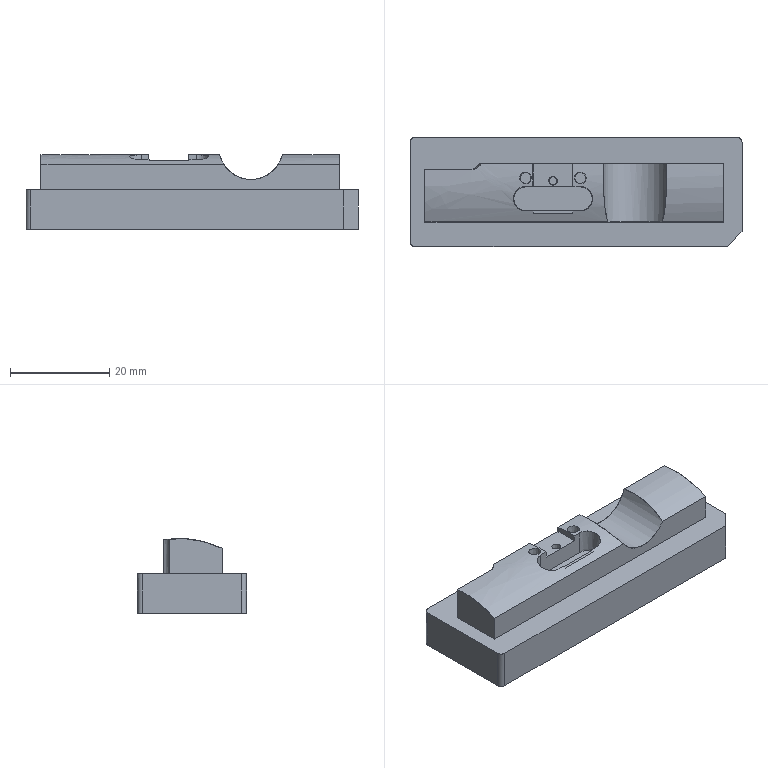NC program | PowerMill | posted with a generic post | part box 67 x 22 x 15.086 mm
Lines 1 to 1040 of 148586:
%
O0001
N104 ( POWERMILL CB  : 2026004.0)
N105 ( POST VER      : 2026.0.0.5161)
N106 ( OPTION FILE   : FANUC)
N107 ( OUTPUT WORKPLANE : WORLD)
N108 (  )
N109 ( TOOL LIST )
N110 (---------------------------------------)
N111 ( NO. | ID        | DIA.| TIP RAD|LENGTH)
N112 (---------------------------------------)
N113 (    1|D10C_1_1   |10.0 |  0.0   |70.52 )
N114 (   15|D3C_2_1    | 3.0 |  0.0   |62.16 )
N115 (   27|D1C_2_1    | 1.0 |  0.0   |60.24 )
N116 (    3|D10_1_1    |10.0 |  0.0   |70.24 )
N117 (   22|R1.5_1_1   | 3.0 |  1.5   |60.28 )
N118 (   10|D3_1_1_1_2 | 3.0 |  0.0   | 62.2 )
N119 (    8|D1_1_1     | 1.0 |  0.0   |60.28 )
N120 (   13|TEXT_D4_1_1| 4.0 |  0.3   |62.36 )
N121 (---------------------------------------)
N122 (  )
N123 ( NUMBER OF TOOLPATHS: 17.0 )
N124 ( ESTIMATED PROGRAM DURATION: 0 HOURS 22 MIN 14 SEC)
N125 (  )
N126 G00 G21 G80 G40 G17
N127 G90
N128 G54
N129 G53 Z0.0
N130 (---------------)
N131 ( START TOOLPATH : 粗公开粗01-扫面平行-D10C )
N132 (---------------)
N133 ( TOOL NO.    :1 )
N134 ( TOOL TYPE   : ENDMILL)
N135 ( TOOL ID     : D10C_1_1)
N136 ( TOOL DIA    : 10.0 LENGTH 70.52)
N137 T1
N138 M6
N139 S8000 M03
N140 G00 G90 X0.0 Y0.0
N141 G43 Z10.2 H1
N142
N143 G05 P10000 R4
N144 X41.15 Y13.65
N145 Z1.1975
N146 G01 Z-0.0025 F6000.0
N147 X36.15 F10000.0
N148 X-36.15
N149 Y8.19
N150 X36.15
N151 Y2.73
N152 X-36.15
N153 Y-2.73
N154 X36.15
N155 Y-8.19
N156 X-36.15
N157 Y-13.65
N158 X36.15
N159 X41.15
N160 Z-0.205
N161 X36.15
N162 X-36.15
N163 Y-8.19
N164 X36.15
N165 Y-2.73
N166 X-36.15
N167 Y2.73
N168 X36.15
N169 Y8.19
N170 X-36.15
N171 Y13.65
N172 X36.15
N173 X41.15
N174 G00 Z10.2
N175 G05 P0
N176 (---------------)
N177 ( END TOOLPATH : 粗公开粗01-扫面平行-D10C )
N178 (---------------)
N179 ( START TOOLPATH : 粗公开粗01-外形偏置-D10C )
N180 (---------------)
N181 G00 X-0.3595 Y-0.0315 Z9.7955
N182 G05 P10000 R4
N183 X42.682 Y10.5169
N184 Z0.6351
N185 G01 Z-0.5649 F6000.0
N186 X42.1545 F10000.0
N187 G03 X37.407 Y5.7694 I0.0 J-4.7475
N188 G01 Y-12.713
N189 G02 X36.407 Y-13.713 I-1.0 J0.0
N190 G01 X-4.6615
N191 Y-9.213
N192 Y-13.713
N193 X-37.126
N194 G02 X-38.126 Y-12.713 I0.0 J1.0
N195 G01 Y12.65
N196 G02 X-37.126 Y13.65 I1.0 J0.0
N197 G01 X36.407
N198 G02 X37.407 Y12.65 I0.0 J-1.0
N199 G01 Y5.7694
N200 X34.9091 Y5.7692
N201 X34.9095 Y-0.4182
N202 X34.902 Y-1.1916
N203 X34.8314 Y-1.8088
N204 X34.5777 Y-2.7385
N205 X34.2095 Y-3.5119
N206 X34.058 Y-3.7528
N207 X33.6575 Y-4.2853
N208 X33.2846 Y-4.6749
N209 X32.8237 Y-5.0588
N210 X32.5111 Y-5.273
N211 X31.7377 Y-5.6689
N212 X31.2876 Y-5.8322
N213 X30.9643 Y-5.9218
N214 X30.1908 Y-6.0524
N215 X29.4174 Y-6.0514
N216 X28.644 Y-6.0081
N217 X22.4566 Y-6.0108
N218 X22.4537
N219 X17.816 Y-6.0659
N220 X17.0426 Y-5.9479
N221 X16.2692 Y-5.7099
N222 X15.4957 Y-5.3238
N223 X15.101 Y-5.0588
N224 X14.7223 Y-4.747
N225 X14.2769 Y-4.2853
N226 X13.9489 Y-3.8691
N227 X13.7229 Y-3.5119
N228 X13.3569 Y-2.7385
N229 X13.1755 Y-2.1508
N230 X13.0336 Y-1.1916
N231 X13.0168 Y-0.4182
N232 X13.0199 Y5.7692
N233 X13.0201 Y5.7722
N234 X10.7908 Y5.7692
N235 X10.7971 Y1.1286
N236 X10.7768 Y-1.1916
N237 X10.6755 Y-1.9651
N238 X10.4515 Y-2.7385
N239 X10.0818 Y-3.5197
N240 X9.5319 Y-4.2853
N241 X9.3083 Y-4.5323
N242 X8.5349 Y-5.1785
N243 X7.7615 Y-5.6129
N244 X7.1733 Y-5.8322
N245 X6.9881 Y-5.8926
N246 X6.2146 Y-6.039
N247 X5.4412 Y-6.0733
N248 X3.1209 Y-6.0724
N249 X2.3475 Y-5.9868
N250 X1.7218 Y-5.8322
N251 X0.8006 Y-5.4335
N252 X0.0272 Y-4.9161
N253 X-0.6151 Y-4.2853
N254 X-0.6631 Y-4.2274
N255 G03 X-0.9979 Y-4.049 I-0.385 J-0.319
N256 G01 X-1.5196 Y-3.9963
N257 X-2.2931 Y-3.7998
N258 X-2.9778 Y-3.5119
N259 X-3.8399 Y-2.9592
N260 X-4.1006 Y-2.7385
N261 X-4.2919 Y-2.5355
N262 G03 X-4.999 Y-2.5149 I-0.3639 J-0.343
N263 G01 X-5.3868 Y-2.8809
N264 X-6.1602 Y-3.4124
N265 X-6.9336 Y-3.7663
N266 X-7.7071 Y-3.9745
N267 X-8.2974 Y-4.0446
N268 G03 X-8.6235 Y-4.2222 I0.059 J-0.4965
N269 G01 X-8.6758 Y-4.2853
N270 X-9.2539 Y-4.8636
N271 X-9.5052 Y-5.0588
N272 X-10.0273 Y-5.3961
N273 X-10.8008 Y-5.7558
N274 X-11.5742 Y-5.977
N275 X-12.3476 Y-6.0711
N276 X-22.4022 Y-6.0455
N277 X-29.363 Y-6.0403
N278 X-30.9098 Y-6.0527
N279 X-31.6833 Y-5.9206
N280 X-32.014 Y-5.8322
N281 X-32.4567 Y-5.6676
N282 X-33.2301 Y-5.2723
N283 X-33.5386 Y-5.0588
N284 X-34.0036 Y-4.6734
N285 X-34.3712 Y-4.2853
N286 X-34.777 Y-3.755
N287 X-34.9267 Y-3.5119
N288 X-35.2947 Y-2.7385
N289 X-35.518 Y-1.9651
N290 X-35.6189 Y-1.1916
N291 X-35.6268 Y4.2223
N292 X-35.6035 Y4.9958
N293 X-35.5504 Y5.391
N294 X-35.4698 Y5.7692
N295 X-35.2075 Y6.5426
N296 X-34.7935 Y7.3161
N297 X-34.177 Y8.0895
N298 X-34.0036 Y8.2604
N299 X-33.2301 Y8.8597
N300 X-32.4567 Y9.2617
N301 X-31.6833 Y9.5142
N302 X-30.9437 Y9.6363
N303 X-30.1364 Y9.6575
N304 X-22.6114
N305 X-22.4647 Y9.6796
N306 X-22.3309 Y9.7437
N307 X-21.6287 Y10.2196
N308 X-21.2529 Y10.4098
N309 X-20.8553 Y10.568
N310 X-20.0819 Y10.7731
N311 X-19.3084 Y10.8552
N312 X-10.0273 Y10.8575
N313 X-8.4805 Y10.8536
N314 X-7.7071 Y10.7648
N315 X-6.9336 Y10.5524
N316 X-6.5839 Y10.4098
N317 X-6.1602 Y10.1987
N318 X-5.3868 Y9.6623
N319 X-4.9839 Y9.2936
N320 G03 X-4.288 Y9.3138 I0.3376 J0.3689
N321 G01 X-3.9741 Y9.6363
N322 X-3.8399 Y9.7461
N323 X-3.0665 Y10.2523
N324 X-2.7447 Y10.4098
N325 X-2.2931 Y10.5865
N326 X-1.5196 Y10.7826
N327 X-0.7462 Y10.8565
N328 X5.4412 Y10.8575
N329 X6.2146 Y10.8253
N330 X6.9881 Y10.6781
N331 X7.7416 Y10.4098
N332 X8.5349 Y9.9667
N333 X8.971 Y9.6363
N334 X9.3083 Y9.3226
N335 X9.7115 Y8.8629
N336 X10.0818 Y8.3149
N337 X10.2073 Y8.0895
N338 X10.5336 Y7.3161
N339 X10.7231 Y6.5426
N340 X10.7908 Y5.7692
N341 X13.0201 Y5.7722
N342 X13.0877 Y6.5426
N343 X13.1755 Y6.9645
N344 X13.2771 Y7.3161
N345 X13.6034 Y8.0895
N346 X13.9489 Y8.6575
N347 X14.0993 Y8.8629
N348 X14.7223 Y9.5329
N349 X15.4957 Y10.1085
N350 X16.2692 Y10.4935
N351 X17.0426 Y10.7327
N352 X17.816 Y10.8431
N353 X18.5894 Y10.8575
N354 X29.4174
N355 X30.1908 Y10.8394
N356 X30.9643 Y10.7146
N357 X31.7377 Y10.4624
N358 X32.5111 Y10.0608
N359 X33.0892 Y9.6363
N360 X33.2846 Y9.462
N361 X33.8296 Y8.8629
N362 X34.058 Y8.544
N363 X34.3255 Y8.0895
N364 X34.6519 Y7.3161
N365 X34.8314 Y6.601
N366 X34.9091 Y5.7692
N367 X37.407 Y5.7694
N368 G00 Z3.3752
N369 G01 X42.682 Y10.5169
N370 G00 Z0.3252
N371 G01 Z-0.8748 F6000.0
N372 X42.1545 F10000.0
N373 G03 X37.407 Y5.7694 I0.0 J-4.7475
N374 G01 Y5.7693
N375 X34.9091 Y5.7692
N376 X34.9093 Y2.0706
N377 X34.9094 Y-0.4182
N378 Y-0.4219
N379 X34.9095 Y-1.9651
N380 X34.8916 Y-2.7385
N381 X34.8314 Y-3.207
N382 X34.7668 Y-3.5119
N383 X34.5157 Y-4.2853
N384 X34.116 Y-5.0588
N385 X33.5168 Y-5.8322
N386 X33.2846 Y-6.068
N387 X32.5971 Y-6.6056
N388 X31.7377 Y-7.0685
N389 X30.9643 Y-7.3208
N390 X30.6654 Y-7.3791
N391 X30.1908 Y-7.4432
N392 X28.644 Y-7.4283
N393 X22.4566 Y-7.4306
N394 X22.4547
N395 X17.816 Y-7.4676
N396 X17.0426 Y-7.3692
N397 X16.2692 Y-7.1465
N398 X15.4957 Y-6.7804
N399 X15.2212 Y-6.6056
N400 X14.7223 Y-6.2304
N401 X14.3092 Y-5.8322
N402 X13.9489 Y-5.4021
N403 X13.715 Y-5.0588
N404 X13.317 Y-4.2853
N405 X13.1755 Y-3.9008
N406 X13.0677 Y-3.5119
N407 X12.9462 Y-2.7385
N408 X12.9179 Y-1.9651
N409 X12.9181 Y4.2223
N410 X12.9141 Y5.7532
N411 X10.8966 Y5.7692
N412 X10.8905 Y4.9958
N413 X10.8922 Y-1.9651
N414 X10.864 Y-2.7385
N415 X10.7422 Y-3.5119
N416 X10.4904 Y-4.2853
N417 X10.0818 Y-5.0809
N418 X9.499 Y-5.8322
N419 X9.3083 Y-6.0291
N420 X8.5875 Y-6.6056
N421 X7.7615 Y-7.0549
N422 X6.9881 Y-7.3168
N423 X6.7042 Y-7.3791
N424 X6.2146 Y-7.4503
N425 X5.4412 Y-7.4734
N426 X3.1209 Y-7.472
N427 X2.3475 Y-7.4118
N428 X1.5741 Y-7.2306
N429 X0.8006 Y-6.9135
N430 X0.0272 Y-6.4409
N431 X-0.7462 Y-5.7134
N432 X-1.2329 Y-5.0588
N433 X-1.5196 Y-4.5318
N434 X-1.6599 Y-4.1825
N435 G03 X-1.9896 Y-3.8871 I-0.464 J-0.1863
N436 G01 X-2.2931 Y-3.8026
N437 X-2.9826 Y-3.5119
N438 X-3.8399 Y-2.9615
N439 X-4.1029 Y-2.7385
N440 X-4.2909 Y-2.5388
N441 G03 X-4.9983 Y-2.5178 I-0.3641 J-0.3426
N442 G01 X-5.3868 Y-2.8846
N443 X-6.1602 Y-3.4163
N444 X-6.9336 Y-3.7695
N445 X-7.2951 Y-3.8753
N446 G03 X-7.6232 Y-4.1805 I0.1405 J-0.4799
N447 G01 X-7.6622 Y-4.2853
N448 X-8.0571 Y-5.0588
N449 X-8.4805 Y-5.6386
N450 X-8.6556 Y-5.8322
N451 X-9.2539 Y-6.3874
N452 X-10.0273 Y-6.88
N453 X-10.8008 Y-7.21
N454 X-11.4341 Y-7.3791
N455 X-12.3476 Y-7.4716
N456 X-17.7616 Y-7.4491
N457 X-29.363 Y-7.4299
N458 X-30.9098 Y-7.4433
N459 X-31.6833 Y-7.3204
N460 X-32.4567 Y-7.0677
N461 X-33.2301 Y-6.6652
N462 X-34.0036 Y-6.0664
N463 X-34.2347 Y-5.8322
N464 X-34.777 Y-5.1473
N465 X-35.233 Y-4.2853
N466 X-35.4849 Y-3.5119
N467 X-35.609 Y-2.7385
N468 X-35.6268 Y-1.9651
N469 Y4.2223
N470 X-35.6035 Y4.9958
N471 X-35.5504 Y5.391
N472 X-35.4698 Y5.7692
N473 X-35.2075 Y6.5426
N474 X-34.7935 Y7.3161
N475 X-34.177 Y8.0895
N476 X-34.0036 Y8.2604
N477 X-33.2301 Y8.8597
N478 X-32.4567 Y9.2617
N479 X-31.6833 Y9.5142
N480 X-30.9437 Y9.6363
N481 X-30.1364 Y9.6575
N482 X-22.6283
N483 X-22.4813 Y9.6796
N484 X-22.3473 Y9.744
N485 X-21.6287 Y10.2321
N486 X-21.2696 Y10.4098
N487 X-20.8553 Y10.5737
N488 X-20.0819 Y10.776
N489 X-19.3084 Y10.8557
N490 X-10.0273 Y10.8575
N491 X-8.4805 Y10.8537
N492 X-7.7071 Y10.765
N493 X-6.9336 Y10.5529
N494 X-6.5808 Y10.4098
N495 X-6.1602 Y10.1997
N496 X-5.3868 Y9.6652
N497 X-4.9844 Y9.295
N498 G03 X-4.2876 Y9.3143 I0.3385 J0.368
N499 G01 X-3.9741 Y9.6363
N500 X-3.8399 Y9.7461
N501 X-3.0665 Y10.2523
N502 X-2.7447 Y10.4098
N503 X-2.2931 Y10.5865
N504 X-1.5196 Y10.7826
N505 X-0.7462 Y10.8565
N506 X5.4412 Y10.8575
N507 X6.2146 Y10.835
N508 X6.9881 Y10.7046
N509 X7.7615 Y10.4461
N510 X8.5349 Y10.0363
N511 X9.0767 Y9.6363
N512 X9.3083 Y9.4271
N513 X9.8176 Y8.8629
N514 X10.0818 Y8.4876
N515 X10.3131 Y8.0895
N516 X10.6394 Y7.3161
N517 X10.8289 Y6.5426
N518 X10.8966 Y5.7692
N519 X12.9141 Y5.7532
N520 Y5.7692
N521 X12.9819 Y6.5426
N522 X13.1714 Y7.3161
N523 X13.4975 Y8.0895
N524 X13.9489 Y8.8032
N525 X14.7223 Y9.6264
N526 X15.4957 Y10.1711
N527 X15.9632 Y10.4098
N528 X16.2692 Y10.5339
N529 X17.0426 Y10.7542
N530 X17.816 Y10.8515
N531 X18.5894 Y10.8575
N532 X29.4174
N533 X30.1908 Y10.8394
N534 X30.9643 Y10.7146
N535 X31.7377 Y10.4624
N536 X32.5111 Y10.0608
N537 X33.0892 Y9.6363
N538 X33.2846 Y9.462
N539 X33.8296 Y8.8629
N540 X34.058 Y8.544
N541 X34.3255 Y8.0895
N542 X34.6519 Y7.3161
N543 X34.8314 Y6.601
N544 X34.9091 Y5.7692
N545 X37.407 Y5.7693
N546 Y-12.713
N547 G02 X36.407 Y-13.713 I-1.0 J0.0
N548 G01 X-37.126
N549 G02 X-38.126 Y-12.713 I0.0 J1.0
N550 G01 Y12.65
N551 G02 X-37.126 Y13.65 I1.0 J0.0
N552 G01 X36.407
N553 G02 X37.407 Y12.65 I0.0 J-1.0
N554 G01 Y5.7694
N555 G00 Z3.0653
N556 G01 X42.682 Y10.5169
N557 G00 Z0.0153
N558 G01 Z-1.1847 F6000.0
N559 X42.1545 F10000.0
N560 G03 X37.407 Y5.7694 I0.0 J-4.7475
N561 G01 Y5.7687
N562 X34.9091 Y5.7692
N563 X34.909 Y5.5281
N564 X34.9092 Y2.0706
N565 X34.9094 Y-0.4182
N566 Y-0.4219
N567 Y-1.9651
N568 X34.9076 Y-2.0433
N569 X34.9074 Y-3.5119
N570 X34.8314 Y-4.2796
N571 X34.6301 Y-5.0588
N572 X34.2915 Y-5.8322
N573 X34.058 Y-6.2197
N574 X33.7768 Y-6.6056
N575 X33.2846 Y-7.1406
N576 X33.012 Y-7.3791
N577 X32.5111 Y-7.7394
N578 X31.7071 Y-8.1525
N579 X30.9643 Y-8.3932
N580 X30.1908 Y-8.517
N581 X17.816 Y-8.5325
N582 X17.0426 Y-8.4525
N583 X16.2692 Y-8.2483
N584 X15.4957 Y-7.9062
N585 X14.7223 Y-7.387
N586 X13.9464 Y-6.6056
N587 X13.4325 Y-5.8322
N588 X13.1755 Y-5.2828
N589 X13.0938 Y-5.0588
N590 X12.8926 Y-4.2853
N591 X12.8097 Y-3.5119
N592 X12.8062 Y-2.7385
N593 X12.8116 Y4.2223
N594 X12.808 Y5.7687
N595 X11.0043 Y5.7692
N596 X11.0016 Y-3.5119
N597 X10.9187 Y-4.2853
N598 X10.7181 Y-5.0588
N599 X10.3789 Y-5.8322
N600 X10.0818 Y-6.3179
N601 X9.8656 Y-6.6056
N602 X9.3083 Y-7.2001
N603 X9.0981 Y-7.3791
N604 X8.5349 Y-7.7793
N605 X7.792 Y-8.1525
N606 X6.9881 Y-8.4077
N607 X6.2146 Y-8.5185
N608 X2.3475 Y-8.5338
N609 X1.5741 Y-8.4902
N610 X0.8006 Y-8.325
N611 X0.0272 Y-8.0304
N612 X-0.7462 Y-7.5736
N613 X-1.5196 Y-6.8894
N614 X-1.7538 Y-6.6056
N615 X-2.2707 Y-5.8322
N616 X-2.6045 Y-5.0588
N617 X-2.8054 Y-4.2853
N618 X-2.8511 Y-3.8329
N619 G03 X-3.0745 Y-3.465 I-0.4975 J-0.0502
N620 G01 X-3.8399 Y-2.9633
N621 X-4.1047 Y-2.7385
N622 X-4.2897 Y-2.5417
N623 G03 X-4.9973 Y-2.5206 I-0.3643 J-0.3425
N624 G01 X-5.3868 Y-2.8884
N625 X-6.1602 Y-3.4197
N626 X-6.1671 Y-3.4233
N627 G03 X-6.4319 Y-3.815 I0.2326 J-0.4426
N628 G01 X-6.48 Y-4.2853
N629 X-6.6818 Y-5.0588
N630 X-7.0209 Y-5.8322
N631 X-7.5341 Y-6.6056
N632 X-7.7071 Y-6.8087
N633 X-8.2994 Y-7.3791
N634 X-8.4805 Y-7.518
N635 X-9.2539 Y-7.9992
N636 X-9.5968 Y-8.1525
N637 X-10.0273 Y-8.3074
N638 X-10.8008 Y-8.4834
N639 X-11.5742 Y-8.5386
N640 X-30.9098 Y-8.517
N641 X-31.6833 Y-8.3928
N642 X-32.4567 Y-8.1398
N643 X-33.2301 Y-7.7383
N644 X-33.7288 Y-7.3791
N645 X-34.0036 Y-7.1391
N646 X-34.4956 Y-6.6056
N647 X-34.777 Y-6.2168
N648 X-35.0078 Y-5.8322
N649 X-35.3472 Y-5.0588
N650 X-35.5474 Y-4.2853
N651 X-35.6242 Y-3.5119
N652 X-35.6247 Y-2.0542
N653 X-35.6267 Y-1.9651
N654 Y4.0618
N655 X-35.6268 Y4.2223
N656 X-35.6035 Y4.9958
N657 X-35.5504 Y5.391
N658 X-35.4698 Y5.7692
N659 X-35.2075 Y6.5426
N660 X-34.7935 Y7.3161
N661 X-34.177 Y8.0895
N662 X-34.0036 Y8.2604
N663 X-33.2301 Y8.8597
N664 X-32.4567 Y9.2617
N665 X-31.6833 Y9.5142
N666 X-30.9437 Y9.6363
N667 X-30.1364 Y9.6575
N668 X-22.6439
N669 X-22.4974 Y9.6795
N670 X-22.3638 Y9.7434
N671 X-21.6287 Y10.2407
N672 X-21.2859 Y10.4098
N673 X-20.8553 Y10.5793
N674 X-20.0819 Y10.7789
N675 X-19.3084 Y10.8561
N676 X-10.0273 Y10.8575
N677 X-8.4805 Y10.8538
N678 X-7.7071 Y10.7653
N679 X-6.9336 Y10.5534
N680 X-6.5776 Y10.4098
N681 X-6.1602 Y10.2004
N682 X-5.3868 Y9.6681
N683 X-5.1713 Y9.4796
N684 X-5.0894 Y9.3916
N685 X-4.9844 Y9.295
N686 G03 X-4.3094 Y9.2932 I0.3385 J0.368
N687 G01 X-4.3021 Y9.3002
N688 X-4.2949 Y9.3074
N689 X-3.9741 Y9.6363
N690 X-3.8399 Y9.7462
N691 X-3.0665 Y10.2524
N692 X-2.7448 Y10.4098
N693 X-2.2931 Y10.5866
N694 X-1.5196 Y10.7827
N695 X-0.7462 Y10.8565
N696 X5.4412 Y10.8575
N697 X6.2146 Y10.8448
N698 X6.9881 Y10.7311
N699 X7.7615 Y10.4918
N700 X8.5349 Y10.1042
N701 X9.1846 Y9.6363
N702 X9.9237 Y8.8629
N703 X10.0818 Y8.6476
N704 X10.4197 Y8.0895
N705 X10.7467 Y7.3161
N706 X10.8552 Y6.9347
N707 X10.9349 Y6.5426
N708 X11.0043 Y5.7692
N709 X12.808 Y5.7687
N710 Y5.7692
N711 X12.8754 Y6.5426
N712 X13.0646 Y7.3161
N713 X13.1755 Y7.6201
N714 X13.3915 Y8.0895
N715 X13.886 Y8.8629
N716 X14.6274 Y9.6363
N717 X15.4957 Y10.2311
N718 X15.8572 Y10.4098
N719 X16.2692 Y10.5744
N720 X17.0426 Y10.7756
N721 X17.816 Y10.8556
N722 X18.3645 Y10.8557
N723 X18.5894 Y10.8575
N724 X29.0893
N725 X29.4174
N726 X30.1908 Y10.8395
N727 X30.9643 Y10.7146
N728 X31.7377 Y10.4624
N729 X32.5111 Y10.0608
N730 X33.0892 Y9.6363
N731 X33.2846 Y9.462
N732 X33.8297 Y8.8629
N733 X34.058 Y8.544
N734 X34.3255 Y8.0895
N735 X34.6519 Y7.3161
N736 X34.8314 Y6.601
N737 X34.9091 Y5.7692
N738 X37.407 Y5.7687
N739 Y-12.713
N740 G02 X36.407 Y-13.713 I-1.0 J0.0
N741 G01 X-37.126
N742 G02 X-38.126 Y-12.713 I0.0 J1.0
N743 G01 Y12.65
N744 G02 X-37.126 Y13.65 I1.0 J0.0
N745 G01 X36.407
N746 G02 X37.407 Y12.65 I0.0 J-1.0
N747 G01 Y5.7694
N748 G00 Z2.7554
N749 G01 X42.682 Y10.5169
N750 G00 Z-0.2946
N751 G01 Z-1.4946 F6000.0
N752 X42.1545 F10000.0
N753 G03 X37.407 Y5.7694 I0.0 J-4.7475
N754 G01 Y5.7693
N755 X34.9091 Y5.7692
N756 X34.9092 Y2.2259
N757 Y2.0706
N758 X34.9093 Y-0.4182
N759 Y-0.4219
N760 X34.9094 Y-1.9651
N761 X34.9093 Y-1.9708
N762 Y-4.2853
N763 X34.8441 Y-5.0588
N764 X34.6584 Y-5.8322
N765 X34.336 Y-6.6056
N766 X34.058 Y-7.0811
N767 X33.8466 Y-7.3791
N768 X33.2846 Y-7.9991
N769 X33.1142 Y-8.1525
N770 X32.5111 Y-8.5988
N771 X31.9085 Y-8.9259
N772 X31.7377 Y-9.0012
N773 X30.9643 Y-9.2524
N774 X30.1908 Y-9.378
N775 X17.816 Y-9.4172
N776 X17.0426 Y-9.357
N777 X16.2692 Y-9.1731
N778 X15.4957 Y-8.8587
N779 X14.7223 Y-8.3746
N780 X14.4503 Y-8.1525
N781 X13.9489 Y-7.6542
N782 X13.7273 Y-7.3791
N783 X13.2407 Y-6.6056
N784 X12.9229 Y-5.8322
N785 X12.7368 Y-5.0588
N786 X12.6643 Y-4.2853
N787 X12.6658 Y5.7692
N788 Y5.7693
N789 X11.1449 Y5.7692
N790 X11.1458 Y-4.2853
N791 X11.0742 Y-5.0588
N792 X10.8878 Y-5.8322
N793 X10.5686 Y-6.6056
N794 X10.0818 Y-7.3833
N795 X9.3588 Y-8.1525
N796 X8.5349 Y-8.7389
N797 X8.1692 Y-8.9259
N798 X7.7615 Y-9.0987
N799 X6.9881 Y-9.3167
N800 X6.2146 Y-9.4087
N801 X-0.7462 Y-9.4149
N802 X-1.5196 Y-9.3402
N803 X-2.2931 Y-9.1434
N804 X-3.0665 Y-8.8085
N805 X-3.8399 Y-8.3013
N806 X-4.0165 Y-8.1525
N807 X-4.2853 Y-7.8739
N808 G03 X-4.989 Y-7.8582 I-0.3598 J-0.3472
N809 G01 X-5.2996 Y-8.1525
N810 X-6.1602 Y-8.7594
N811 X-6.9336 Y-9.1121
N812 X-7.7071 Y-9.3238
N813 X-8.4805 Y-9.4121
N814 X-27.0427 Y-9.4125
N815 X-30.9098 Y-9.3932
N816 X-31.6833 Y-9.2681
N817 X-32.4567 Y-9.0144
N818 X-33.2301 Y-8.6122
N819 X-34.0036 Y-8.0133
N820 X-34.5736 Y-7.3791
N821 X-34.777 Y-7.0945
N822 X-35.0608 Y-6.6056
N823 X-35.38 Y-5.8322
N824 X-35.5504 Y-5.1449
N825 X-35.6267 Y-4.2853
N826 X-35.6268 Y4.2223
N827 X-35.6035 Y4.9958
N828 X-35.5504 Y5.391
N829 X-35.4698 Y5.7692
N830 X-35.2076 Y6.5426
N831 X-34.7935 Y7.3161
N832 X-34.177 Y8.0895
N833 X-34.0036 Y8.2604
N834 X-33.2301 Y8.8597
N835 X-32.4567 Y9.2617
N836 X-31.6833 Y9.5142
N837 X-30.9437 Y9.6363
N838 X-30.1364 Y9.6575
N839 X-22.6596
N840 X-22.5135 Y9.6794
N841 X-22.3802 Y9.7429
N842 X-21.6287 Y10.2492
N843 X-21.3022 Y10.4098
N844 X-20.8553 Y10.5849
N845 X-20.0819 Y10.7818
N846 X-19.3084 Y10.8564
N847 X-10.0273 Y10.8575
N848 X-8.4805 Y10.8539
N849 X-7.7071 Y10.7656
N850 X-6.9336 Y10.554
N851 X-6.5759 Y10.4098
N852 X-6.1602 Y10.2034
N853 X-5.8067 Y9.9571
N854 X-5.3868 Y9.6681
N855 X-5.366 Y9.6499
N856 X-5.3466 Y9.6363
N857 X-5.1693 Y9.4789
N858 X-5.0795 Y9.3824
N859 X-4.9844 Y9.295
N860 G03 X-4.3851 Y9.2363 I0.3385 J0.368
N861 G01 X-4.3387 Y9.2696
N862 X-4.2964 Y9.3081
N863 X-3.9742 Y9.6363
N864 X-3.8399 Y9.7462
N865 X-3.0665 Y10.2524
N866 X-2.7448 Y10.4098
N867 X-2.2931 Y10.5866
N868 X-1.5196 Y10.7827
N869 X-0.7462 Y10.8566
N870 X5.4412 Y10.8575
N871 X6.2146 Y10.8528
N872 X6.9881 Y10.7606
N873 X7.7615 Y10.5447
N874 X8.0957 Y10.4098
N875 X8.5349 Y10.1873
N876 X9.325 Y9.6363
N877 X10.0654 Y8.8629
N878 X10.5613 Y8.0895
N879 X10.8552 Y7.411
N880 X11.0771 Y6.5426
N881 X11.1449 Y5.7692
N882 X12.6658 Y5.7693
N883 X12.7336 Y6.5426
N884 X12.9231 Y7.3161
N885 X13.2492 Y8.0895
N886 X13.7451 Y8.8629
N887 X13.9489 Y9.1084
N888 X14.4851 Y9.6363
N889 X14.7223 Y9.8249
N890 X15.4957 Y10.305
N891 X16.2692 Y10.6192
N892 X17.0426 Y10.7984
N893 X17.816 Y10.8575
N894 X29.4174
N895 X30.1908 Y10.8395
N896 X30.9643 Y10.7146
N897 X31.7377 Y10.4624
N898 X32.5111 Y10.0608
N899 X33.0892 Y9.6363
N900 X33.2846 Y9.462
N901 X33.8297 Y8.8629
N902 X34.058 Y8.544
N903 X34.3255 Y8.0895
N904 X34.6519 Y7.3161
N905 X34.8314 Y6.601
N906 X34.9091 Y5.7692
N907 X37.407 Y5.7693
N908 Y-12.713
N909 G02 X36.407 Y-13.713 I-1.0 J0.0
N910 G01 X-37.126
N911 G02 X-38.126 Y-12.713 I0.0 J1.0
N912 G01 Y12.65
N913 G02 X-37.126 Y13.65 I1.0 J0.0
N914 G01 X36.407
N915 G02 X37.407 Y12.65 I0.0 J-1.0
N916 G01 Y5.7694
N917 G00 Z2.379
N918 G01 X42.682 Y10.5169
N919 G00 Z-0.671
N920 G01 Z-1.871 F6000.0
N921 X42.1545 F10000.0
N922 G03 X37.407 Y5.7694 I0.0 J-4.7475
N923 G01 Y5.7693
N924 X34.9091 Y5.7692
N925 X34.9095 Y-5.0588
N926 X34.8719 Y-5.8322
N927 X34.8314 Y-6.1143
N928 X34.7188 Y-6.6056
N929 X34.4354 Y-7.3791
N930 X34.058 Y-8.0573
N931 X33.3347 Y-8.9259
N932 X32.5111 Y-9.5741
N933 X32.3012 Y-9.6993
N934 X31.7377 Y-9.9755
N935 X30.9643 Y-10.228
N936 X30.1908 Y-10.3528
N937 X29.4174 Y-10.3705
N938 X17.816 Y-10.3706
N939 X17.0426 Y-10.3344
N940 X16.2692 Y-10.1849
N941 X15.4957 Y-9.9044
N942 X15.1004 Y-9.6993
N943 X14.7223 Y-9.4674
N944 X13.9489 Y-8.8144
N945 X13.4062 Y-8.1525
N946 X13.1755 Y-7.7904
N947 X12.9644 Y-7.3791
N948 X12.6796 Y-6.6056
N949 X12.5254 Y-5.8322
N950 X12.4884 Y-5.0588
N951 X12.4878 Y4.9958
N952 X12.4877 Y4.9986
N953 X12.4792 Y5.7562
N954 X11.3315 Y5.7692
N955 X11.3227 Y4.9958
N956 X11.3228 Y-5.0588
N957 X11.2855 Y-5.8322
N958 X11.1307 Y-6.6056
N959 X10.8552 Y-7.3634
N960 X10.4056 Y-8.1525
N961 X10.0818 Y-8.5739
N962 X9.748 Y-8.9259
N963 X9.3083 Y-9.3078
N964 X8.7095 Y-9.6993
N965 X8.5349 Y-9.7978
N966 X7.7615 Y-10.1192
N967 X6.9881 Y-10.304
N968 X6.2146 Y-10.3685
N969 X-30.1364 Y-10.3704
N970 X-30.9098 Y-10.3524
N971 X-31.6833 Y-10.2272
N972 X-32.4567 Y-9.9747
N973 X-33.2301 Y-9.5727
N974 X-34.0036 Y-8.9737
N975 X-34.7109 Y-8.1525
N976 X-35.1525 Y-7.3791
N977 X-35.4364 Y-6.6056
N978 X-35.589 Y-5.8322
N979 X-35.6268 Y-5.0588
N980 Y4.2223
N981 X-35.6035 Y4.9958
N982 X-35.5504 Y5.391
N983 X-35.4698 Y5.7692
N984 X-35.2076 Y6.5426
N985 X-34.7935 Y7.3161
N986 X-34.177 Y8.0895
N987 X-34.0036 Y8.2604
N988 X-33.2301 Y8.8597
N989 X-32.4567 Y9.2618
N990 X-31.6833 Y9.5142
N991 X-30.9437 Y9.6363
N992 X-30.1364 Y9.6575
N993 X-22.6791
N994 X-22.5336 Y9.6792
N995 X-22.4007 Y9.7422
N996 X-21.6287 Y10.2596
N997 X-21.322 Y10.4098
N998 X-20.8553 Y10.5915
N999 X-20.0819 Y10.7852
N1000 X-19.3084 Y10.8568
N1001 X-15.026 Y10.8569
N1002 X-10.0273 Y10.8575
N1003 X-9.8313 Y10.857
N1004 X4.9863 Y10.8574
N1005 X5.4412 Y10.8575
N1006 X5.4509 Y10.8574
N1007 X6.2146
N1008 X6.9881 Y10.7937
N1009 X7.7615 Y10.6101
N1010 X8.2821 Y10.4098
N1011 X8.5349 Y10.2883
N1012 X9.3083 Y9.7996
N1013 X9.5113 Y9.6363
N1014 X10.0818 Y9.0703
N1015 X10.2517 Y8.8629
N1016 X10.7477 Y8.0895
N1017 X11.0739 Y7.3161
N1018 X11.2634 Y6.5426
N1019 X11.3315 Y5.7692
N1020 X12.4792 Y5.7562
N1021 X12.4791 Y5.7692
N1022 X12.5473 Y6.5426
N1023 X12.7365 Y7.3161
N1024 X13.0627 Y8.0895
N1025 X13.1755 Y8.2939
N1026 X13.559 Y8.8629
N1027 X13.9489 Y9.3098
N1028 X14.2994 Y9.6363
N1029 X14.7223 Y9.9591
N1030 X15.4957 Y10.3946
N1031 X16.2692 Y10.6751
N1032 X17.0426 Y10.8233
N1033 X17.816 Y10.8575
N1034 X29.4174
N1035 X30.1908 Y10.8395
N1036 X30.9643 Y10.7146
N1037 X31.7377 Y10.4624
N1038 X32.5111 Y10.0608
N1039 X33.0892 Y9.6363
N1040 X33.2846 Y9.4621
N1041 X33.8297 Y8.8629
N1042 X34.058 Y8.544
N1043 X34.3255 Y8.0895
N1044 X34.6519 Y7.3161
N1045 X34.8314 Y6.601
N1046 X34.9091 Y5.7692
N1047 X37.407 Y5.7693
N1048 Y-12.713
N1049 G02 X36.407 Y-13.713 I-1.0 J0.0
N1050 G01 X-37.126
N1051 G02 X-38.126 Y-12.713 I0.0 J1.0
N1052 G01 Y12.65
N1053 G02 X-37.126 Y13.65 I1.0 J0.0
N1054 G01 X36.407
N1055 G02 X37.407 Y12.65 I0.0 J-1.0
N1056 G01 Y5.7694
N1057 G00 Z2.0027
N1058 G01 X42.682 Y10.5169
N1059 G00 Z-1.0473
N1060 G01 Z-2.2473 F6000.0
N1061 X42.1545 F10000.0
N1062 G03 X37.407 Y5.7694 I0.0 J-4.7475
N1063 G01 Y5.7693
N1064 X34.9091 Y5.7692
N1065 X34.9093 Y-1.1323
N1066 X34.9094 Y-5.0588
N1067 Y-5.0594
N1068 Y-5.8322
N1069 X34.8809 Y-6.6056
N1070 X34.7387 Y-7.3791
N1071 X34.467 Y-8.1525
N1072 X34.058 Y-8.9004
N1073 X33.4073 Y-9.6993
N1074 X33.2846 Y-9.8185
N1075 X32.4213 Y-10.4728
N1076 X31.7377 Y-10.8189
N1077 X30.9643 Y-11.0711
N1078 X30.1908 Y-11.1959
N1079 X29.4174 Y-11.214
N1080 X17.816
N1081 X17.0426 Y-11.2002
N1082 X16.2692 Y-11.0848
N1083 X15.4957 Y-10.8433
N1084 X14.7519 Y-10.4728
N1085 X13.9489 Y-9.874
N1086 X13.7659 Y-9.6993
N1087 X13.1755 Y-8.9895
N1088 X12.7062 Y-8.1525
N1089 X12.4345 Y-7.3791
N1090 X12.2923 Y-6.6056
N1091 X12.2536 Y-5.8322
N1092 X12.2528 Y5.7692
N1093 X11.5577
N1094 X11.5573 Y-5.8322
N1095 X11.5184 Y-6.6056
N1096 X11.3762 Y-7.3791
N1097 X11.1045 Y-8.1525
N1098 X10.8552 Y-8.6419
N1099 X10.6786 Y-8.9259
N1100 X10.0818 Y-9.6611
N1101 X9.3083 Y-10.3117
N1102 X9.0588 Y-10.4728
N1103 X8.5349 Y-10.7491
N1104 X7.7615 Y-11.0298
N1105 X6.9881 Y-11.176
N1106 X6.2146 Y-11.214
N1107 X-30.1364
N1108 X-30.9098 Y-11.1957
N1109 X-31.6833 Y-11.0707
N1110 X-32.4567 Y-10.8182
N1111 X-33.1386 Y-10.4728
N1112 X-34.0036 Y-9.8168
N1113 X-34.1246 Y-9.6993
N1114 X-34.7583 Y-8.9259
N1115 X-35.1842 Y-8.1525
N1116 X-35.456 Y-7.3791
N1117 X-35.5981 Y-6.6056
N1118 X-35.6268 Y-5.8322
N1119 Y4.2223
N1120 X-35.6035 Y4.9958
N1121 X-35.6033 Y4.9972
N1122 X-35.5504 Y5.391
N1123 X-35.47 Y5.7678
N1124 X-35.4698 Y5.7692
N1125 X-35.2076 Y6.5426
N1126 X-34.7935 Y7.3161
N1127 X-34.177 Y8.0895
N1128 X-34.0036 Y8.2604
N1129 X-33.2301 Y8.8597
N1130 X-32.4567 Y9.2618
N1131 X-31.6833 Y9.5142
N1132 X-30.9437 Y9.6363
N1133 X-30.1364 Y9.6575
N1134 X-22.7213
N1135 X-22.5562 Y9.6856
N1136 X-22.4096 Y9.7665
N1137 X-22.4022 Y9.7725